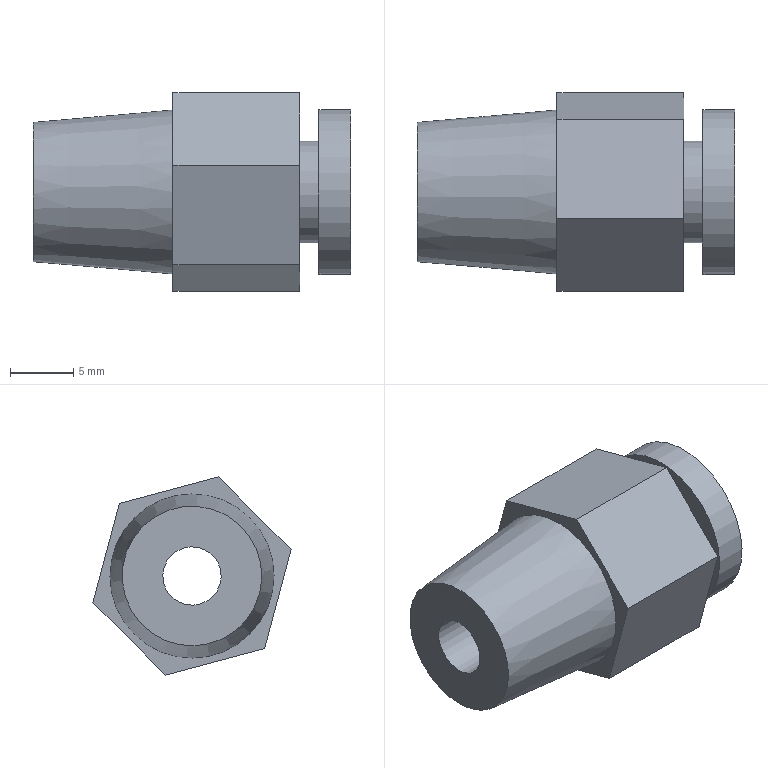Part | NX | features solid 2 | 1 solid | 17 faces | box 25 x 15.612 x 15.618 mm | volume 2729 mm3 | plane 12 | cylinder 4 | cone 1 | commonest cylinder face diameters 4.6 x1 6 x1 8 x1 13 x1
STEP:
#1=CARTESIAN_POINT('',(56.,-265.281,333.212));
#2=VERTEX_POINT('',#1);
#3=CARTESIAN_POINT('',(56.,-273.087,335.309));
#4=VERTEX_POINT('',#3);
#5=CARTESIAN_POINT('',(56.,-265.281,333.212));
#6=DIRECTION('',(0.,-0.9658,0.2594));
#7=VECTOR('',#6,1000.);
#8=LINE('',#5,#7);
#9=EDGE_CURVE('',#2,#4,#8,.T.);
#10=ORIENTED_EDGE('',*,*,#9,.T.);
#11=CARTESIAN_POINT('',(66.,-273.087,335.309));
#12=VERTEX_POINT('',#11);
#13=CARTESIAN_POINT('',(70.,-273.087,335.309));
#14=DIRECTION('',(-1.,0.,0.));
#15=VECTOR('',#14,1000.);
#16=LINE('',#13,#15);
#17=EDGE_CURVE('',#12,#4,#16,.T.);
#18=ORIENTED_EDGE('',*,*,#17,.F.);
#19=CARTESIAN_POINT('',(66.,-265.281,333.212));
#20=VERTEX_POINT('',#19);
#21=CARTESIAN_POINT('',(66.,-265.281,333.212));
#22=DIRECTION('',(0.,-0.9658,0.2594));
#23=VECTOR('',#22,1000.);
#24=LINE('',#21,#23);
#25=EDGE_CURVE('',#20,#12,#24,.T.);
#26=ORIENTED_EDGE('',*,*,#25,.F.);
#27=CARTESIAN_POINT('',(70.,-265.281,333.212));
#28=DIRECTION('',(-1.,0.,0.));
#29=VECTOR('',#28,1000.);
#30=LINE('',#27,#29);
#31=EDGE_CURVE('',#20,#2,#30,.T.);
#32=ORIENTED_EDGE('',*,*,#31,.T.);
#33=EDGE_LOOP('',(#10,#18,#26,#32));
#34=FACE_BOUND('',#33,.T.);
#35=CARTESIAN_POINT('',(70.,-265.281,333.212));
#36=DIRECTION('',(0.,0.2594,0.9658));
#37=DIRECTION('',(0.,-0.9658,0.2594));
#38=AXIS2_PLACEMENT_3D('',#35,#36,#37);
#39=PLANE('',#38);
#40=ADVANCED_FACE('',(#34),#39,.T.);
#41=CARTESIAN_POINT('',(56.,-278.806,329.597));
#42=VERTEX_POINT('',#41);
#43=CARTESIAN_POINT('',(56.,-273.087,335.309));
#44=DIRECTION('',(0.,-0.7076,-0.7066));
#45=VECTOR('',#44,1000.);
#46=LINE('',#43,#45);
#47=EDGE_CURVE('',#4,#42,#46,.T.);
#48=ORIENTED_EDGE('',*,*,#47,.T.);
#49=CARTESIAN_POINT('',(66.,-278.806,329.597));
#50=VERTEX_POINT('',#49);
#51=CARTESIAN_POINT('',(70.,-278.806,329.597));
#52=DIRECTION('',(-1.,0.,0.));
#53=VECTOR('',#52,1000.);
#54=LINE('',#51,#53);
#55=EDGE_CURVE('',#50,#42,#54,.T.);
#56=ORIENTED_EDGE('',*,*,#55,.F.);
#57=CARTESIAN_POINT('',(66.,-273.087,335.309));
#58=DIRECTION('',(0.,-0.7076,-0.7066));
#59=VECTOR('',#58,1000.);
#60=LINE('',#57,#59);
#61=EDGE_CURVE('',#12,#50,#60,.T.);
#62=ORIENTED_EDGE('',*,*,#61,.F.);
#63=ORIENTED_EDGE('',*,*,#17,.T.);
#64=EDGE_LOOP('',(#48,#56,#62,#63));
#65=FACE_BOUND('',#64,.T.);
#66=CARTESIAN_POINT('',(70.,-273.087,335.309));
#67=DIRECTION('',(0.,-0.7066,0.7076));
#68=DIRECTION('',(0.,-0.7076,-0.7066));
#69=AXIS2_PLACEMENT_3D('',#66,#67,#68);
#70=PLANE('',#69);
#71=ADVANCED_FACE('',(#65),#70,.T.);
#72=CARTESIAN_POINT('',(56.,-276.719,321.788));
#73=VERTEX_POINT('',#72);
#74=CARTESIAN_POINT('',(56.,-278.806,329.597));
#75=DIRECTION('',(0.,0.2582,-0.9661));
#76=VECTOR('',#75,1000.);
#77=LINE('',#74,#76);
#78=EDGE_CURVE('',#42,#73,#77,.T.);
#79=ORIENTED_EDGE('',*,*,#78,.T.);
#80=CARTESIAN_POINT('',(66.,-276.719,321.788));
#81=VERTEX_POINT('',#80);
#82=CARTESIAN_POINT('',(70.,-276.719,321.788));
#83=DIRECTION('',(-1.,0.,0.));
#84=VECTOR('',#83,1000.);
#85=LINE('',#82,#84);
#86=EDGE_CURVE('',#81,#73,#85,.T.);
#87=ORIENTED_EDGE('',*,*,#86,.F.);
#88=CARTESIAN_POINT('',(66.,-278.806,329.597));
#89=DIRECTION('',(0.,0.2582,-0.9661));
#90=VECTOR('',#89,1000.);
#91=LINE('',#88,#90);
#92=EDGE_CURVE('',#50,#81,#91,.T.);
#93=ORIENTED_EDGE('',*,*,#92,.F.);
#94=ORIENTED_EDGE('',*,*,#55,.T.);
#95=EDGE_LOOP('',(#79,#87,#93,#94));
#96=FACE_BOUND('',#95,.T.);
#97=CARTESIAN_POINT('',(70.,-278.806,329.597));
#98=DIRECTION('',(0.,-0.9661,-0.2582));
#99=DIRECTION('',(0.,0.2582,-0.9661));
#100=AXIS2_PLACEMENT_3D('',#97,#98,#99);
#101=PLANE('',#100);
#102=ADVANCED_FACE('',(#96),#101,.T.);
#103=CARTESIAN_POINT('',(56.,-268.913,319.691));
#104=VERTEX_POINT('',#103);
#105=CARTESIAN_POINT('',(56.,-276.719,321.788));
#106=DIRECTION('',(0.,0.9658,-0.2594));
#107=VECTOR('',#106,1000.);
#108=LINE('',#105,#107);
#109=EDGE_CURVE('',#73,#104,#108,.T.);
#110=ORIENTED_EDGE('',*,*,#109,.T.);
#111=CARTESIAN_POINT('',(66.,-268.913,319.691));
#112=VERTEX_POINT('',#111);
#113=CARTESIAN_POINT('',(70.,-268.913,319.691));
#114=DIRECTION('',(-1.,0.,0.));
#115=VECTOR('',#114,1000.);
#116=LINE('',#113,#115);
#117=EDGE_CURVE('',#112,#104,#116,.T.);
#118=ORIENTED_EDGE('',*,*,#117,.F.);
#119=CARTESIAN_POINT('',(66.,-276.719,321.788));
#120=DIRECTION('',(0.,0.9658,-0.2594));
#121=VECTOR('',#120,1000.);
#122=LINE('',#119,#121);
#123=EDGE_CURVE('',#81,#112,#122,.T.);
#124=ORIENTED_EDGE('',*,*,#123,.F.);
#125=ORIENTED_EDGE('',*,*,#86,.T.);
#126=EDGE_LOOP('',(#110,#118,#124,#125));
#127=FACE_BOUND('',#126,.T.);
#128=CARTESIAN_POINT('',(70.,-276.719,321.788));
#129=DIRECTION('',(0.,-0.2594,-0.9658));
#130=DIRECTION('',(0.,0.9658,-0.2594));
#131=AXIS2_PLACEMENT_3D('',#128,#129,#130);
#132=PLANE('',#131);
#133=ADVANCED_FACE('',(#127),#132,.T.);
#134=CARTESIAN_POINT('',(56.,-263.194,325.403));
#135=VERTEX_POINT('',#134);
#136=CARTESIAN_POINT('',(56.,-268.913,319.691));
#137=DIRECTION('',(0.,0.7076,0.7066));
#138=VECTOR('',#137,1000.);
#139=LINE('',#136,#138);
#140=EDGE_CURVE('',#104,#135,#139,.T.);
#141=ORIENTED_EDGE('',*,*,#140,.T.);
#142=CARTESIAN_POINT('',(66.,-263.194,325.403));
#143=VERTEX_POINT('',#142);
#144=CARTESIAN_POINT('',(70.,-263.194,325.403));
#145=DIRECTION('',(-1.,0.,0.));
#146=VECTOR('',#145,1000.);
#147=LINE('',#144,#146);
#148=EDGE_CURVE('',#143,#135,#147,.T.);
#149=ORIENTED_EDGE('',*,*,#148,.F.);
#150=CARTESIAN_POINT('',(66.,-268.913,319.691));
#151=DIRECTION('',(0.,0.7076,0.7066));
#152=VECTOR('',#151,1000.);
#153=LINE('',#150,#152);
#154=EDGE_CURVE('',#112,#143,#153,.T.);
#155=ORIENTED_EDGE('',*,*,#154,.F.);
#156=ORIENTED_EDGE('',*,*,#117,.T.);
#157=EDGE_LOOP('',(#141,#149,#155,#156));
#158=FACE_BOUND('',#157,.T.);
#159=CARTESIAN_POINT('',(70.,-268.913,319.691));
#160=DIRECTION('',(0.,0.7066,-0.7076));
#161=DIRECTION('',(0.,0.7076,0.7066));
#162=AXIS2_PLACEMENT_3D('',#159,#160,#161);
#163=PLANE('',#162);
#164=ADVANCED_FACE('',(#158),#163,.T.);
#165=CARTESIAN_POINT('',(56.,-263.194,325.403));
#166=DIRECTION('',(0.,-0.2582,0.9661));
#167=VECTOR('',#166,1000.);
#168=LINE('',#165,#167);
#169=EDGE_CURVE('',#135,#2,#168,.T.);
#170=ORIENTED_EDGE('',*,*,#169,.T.);
#171=ORIENTED_EDGE('',*,*,#31,.F.);
#172=CARTESIAN_POINT('',(66.,-263.194,325.403));
#173=DIRECTION('',(0.,-0.2582,0.9661));
#174=VECTOR('',#173,1000.);
#175=LINE('',#172,#174);
#176=EDGE_CURVE('',#143,#20,#175,.T.);
#177=ORIENTED_EDGE('',*,*,#176,.F.);
#178=ORIENTED_EDGE('',*,*,#148,.T.);
#179=EDGE_LOOP('',(#170,#171,#177,#178));
#180=FACE_BOUND('',#179,.T.);
#181=CARTESIAN_POINT('',(70.,-263.194,325.403));
#182=DIRECTION('',(0.,0.9661,0.2582));
#183=DIRECTION('',(0.,-0.2582,0.9661));
#184=AXIS2_PLACEMENT_3D('',#181,#182,#183);
#185=PLANE('',#184);
#186=ADVANCED_FACE('',(#180),#185,.T.);
#187=ORIENTED_EDGE('',*,*,#25,.T.);
#188=ORIENTED_EDGE('',*,*,#61,.T.);
#189=ORIENTED_EDGE('',*,*,#92,.T.);
#190=ORIENTED_EDGE('',*,*,#123,.T.);
#191=ORIENTED_EDGE('',*,*,#154,.T.);
#192=ORIENTED_EDGE('',*,*,#176,.T.);
#193=EDGE_LOOP('',(#187,#188,#189,#190,#191,#192));
#194=FACE_BOUND('',#193,.T.);
#195=CARTESIAN_POINT('',(66.,-273.83,324.673));
#196=VERTEX_POINT('',#195);
#197=CARTESIAN_POINT('',(66.,-271.,327.5));
#198=DIRECTION('',(-1.,0.,0.));
#199=DIRECTION('',(0.,-0.7076,-0.7066));
#200=AXIS2_PLACEMENT_3D('',#197,#198,#199);
#201=CIRCLE('',#200,4.);
#202=EDGE_CURVE('',#196,#196,#201,.F.);
#203=ORIENTED_EDGE('',*,*,#202,.F.);
#204=EDGE_LOOP('',(#203));
#205=FACE_BOUND('',#204,.T.);
#206=CARTESIAN_POINT('',(66.,-257.475,331.115));
#207=DIRECTION('',(1.,0.,0.));
#208=DIRECTION('',(0.,-0.7076,-0.7066));
#209=AXIS2_PLACEMENT_3D('',#206,#207,#208);
#210=PLANE('',#209);
#211=ADVANCED_FACE('',(#194,#205),#210,.T.);
#212=CARTESIAN_POINT('',(56.,-275.571,322.935));
#213=VERTEX_POINT('',#212);
#214=CARTESIAN_POINT('',(56.,-271.,327.5));
#215=DIRECTION('',(-1.,0.,0.));
#216=DIRECTION('',(0.,-0.7076,-0.7066));
#217=AXIS2_PLACEMENT_3D('',#214,#215,#216);
#218=CIRCLE('',#217,6.46);
#219=EDGE_CURVE('',#213,#213,#218,.F.);
#220=ORIENTED_EDGE('',*,*,#219,.T.);
#221=EDGE_LOOP('',(#220));
#222=FACE_BOUND('',#221,.T.);
#223=ORIENTED_EDGE('',*,*,#9,.F.);
#224=ORIENTED_EDGE('',*,*,#169,.F.);
#225=ORIENTED_EDGE('',*,*,#140,.F.);
#226=ORIENTED_EDGE('',*,*,#109,.F.);
#227=ORIENTED_EDGE('',*,*,#78,.F.);
#228=ORIENTED_EDGE('',*,*,#47,.F.);
#229=EDGE_LOOP('',(#223,#224,#225,#226,#227,#228));
#230=FACE_BOUND('',#229,.T.);
#231=CARTESIAN_POINT('',(56.,-257.475,331.115));
#232=DIRECTION('',(1.,0.,0.));
#233=DIRECTION('',(0.,-0.7076,-0.7066));
#234=AXIS2_PLACEMENT_3D('',#231,#232,#233);
#235=PLANE('',#234);
#236=ADVANCED_FACE('',(#222,#230),#235,.F.);
#237=CARTESIAN_POINT('',(45.,-272.627,325.875));
#238=VERTEX_POINT('',#237);
#239=CARTESIAN_POINT('',(45.,-271.,327.5));
#240=DIRECTION('',(-1.,0.,0.));
#241=DIRECTION('',(0.,-0.7076,-0.7066));
#242=AXIS2_PLACEMENT_3D('',#239,#240,#241);
#243=CIRCLE('',#242,2.3);
#244=EDGE_CURVE('',#238,#238,#243,.T.);
#245=ORIENTED_EDGE('',*,*,#244,.F.);
#246=EDGE_LOOP('',(#245));
#247=FACE_BOUND('',#246,.T.);
#248=CARTESIAN_POINT('',(45.,-267.11,331.385));
#249=VERTEX_POINT('',#248);
#250=CARTESIAN_POINT('',(45.,-271.,327.5));
#251=DIRECTION('',(1.,0.,0.));
#252=DIRECTION('',(0.,0.7076,0.7066));
#253=AXIS2_PLACEMENT_3D('',#250,#251,#252);
#254=CIRCLE('',#253,5.498);
#255=EDGE_CURVE('',#249,#249,#254,.T.);
#256=ORIENTED_EDGE('',*,*,#255,.F.);
#257=EDGE_LOOP('',(#256));
#258=FACE_BOUND('',#257,.T.);
#259=CARTESIAN_POINT('',(45.,-271.,327.5));
#260=DIRECTION('',(-1.,0.,0.));
#261=DIRECTION('',(0.,0.7076,0.7066));
#262=AXIS2_PLACEMENT_3D('',#259,#260,#261);
#263=PLANE('',#262);
#264=ADVANCED_FACE('',(#247,#258),#263,.T.);
#265=ORIENTED_EDGE('',*,*,#255,.T.);
#266=EDGE_LOOP('',(#265));
#267=FACE_BOUND('',#266,.T.);
#268=ORIENTED_EDGE('',*,*,#219,.F.);
#269=EDGE_LOOP('',(#268));
#270=FACE_BOUND('',#269,.T.);
#271=CARTESIAN_POINT('',(45.044,-271.,327.5));
#272=DIRECTION('',(1.,0.,0.));
#273=DIRECTION('',(0.,0.7076,0.7066));
#274=AXIS2_PLACEMENT_3D('',#271,#272,#273);
#275=CONICAL_SURFACE('',#274,5.502,0.08727);
#276=ADVANCED_FACE('',(#267,#270),#275,.T.);
#277=CARTESIAN_POINT('',(53.,-269.373,329.125));
#278=VERTEX_POINT('',#277);
#279=CARTESIAN_POINT('',(53.,-271.,327.5));
#280=DIRECTION('',(1.,0.,0.));
#281=DIRECTION('',(0.,0.7076,0.7066));
#282=AXIS2_PLACEMENT_3D('',#279,#280,#281);
#283=CIRCLE('',#282,2.3);
#284=EDGE_CURVE('',#278,#278,#283,.F.);
#285=ORIENTED_EDGE('',*,*,#284,.F.);
#286=EDGE_LOOP('',(#285));
#287=FACE_BOUND('',#286,.T.);
#288=ORIENTED_EDGE('',*,*,#244,.T.);
#289=EDGE_LOOP('',(#288));
#290=FACE_BOUND('',#289,.T.);
#291=CARTESIAN_POINT('',(45.,-271.,327.5));
#292=DIRECTION('',(1.,0.,0.));
#293=DIRECTION('',(0.,-0.7076,-0.7066));
#294=AXIS2_PLACEMENT_3D('',#291,#292,#293);
#295=CYLINDRICAL_SURFACE('',#294,2.3);
#296=ADVANCED_FACE('',(#287,#290),#295,.F.);
#297=CARTESIAN_POINT('',(53.,-268.877,329.62));
#298=VERTEX_POINT('',#297);
#299=CARTESIAN_POINT('',(53.,-271.,327.5));
#300=DIRECTION('',(1.,0.,0.));
#301=DIRECTION('',(0.,0.7076,0.7066));
#302=AXIS2_PLACEMENT_3D('',#299,#300,#301);
#303=CIRCLE('',#302,3.);
#304=EDGE_CURVE('',#298,#298,#303,.T.);
#305=ORIENTED_EDGE('',*,*,#304,.T.);
#306=EDGE_LOOP('',(#305));
#307=FACE_BOUND('',#306,.T.);
#308=ORIENTED_EDGE('',*,*,#284,.T.);
#309=EDGE_LOOP('',(#308));
#310=FACE_BOUND('',#309,.T.);
#311=CARTESIAN_POINT('',(53.,-271.,327.5));
#312=DIRECTION('',(-1.,0.,0.));
#313=DIRECTION('',(0.,0.7076,0.7066));
#314=AXIS2_PLACEMENT_3D('',#311,#312,#313);
#315=PLANE('',#314);
#316=ADVANCED_FACE('',(#307,#310),#315,.F.);
#317=ORIENTED_EDGE('',*,*,#304,.F.);
#318=EDGE_LOOP('',(#317));
#319=FACE_BOUND('',#318,.T.);
#320=CARTESIAN_POINT('',(70.,-273.123,325.38));
#321=VERTEX_POINT('',#320);
#322=CARTESIAN_POINT('',(70.,-271.,327.5));
#323=DIRECTION('',(1.,0.,0.));
#324=DIRECTION('',(0.,-0.7076,-0.7066));
#325=AXIS2_PLACEMENT_3D('',#322,#323,#324);
#326=CIRCLE('',#325,3.);
#327=EDGE_CURVE('',#321,#321,#326,.T.);
#328=ORIENTED_EDGE('',*,*,#327,.T.);
#329=EDGE_LOOP('',(#328));
#330=FACE_BOUND('',#329,.T.);
#331=CARTESIAN_POINT('',(70.,-271.,327.5));
#332=DIRECTION('',(-1.,0.,0.));
#333=DIRECTION('',(0.,0.7076,0.7066));
#334=AXIS2_PLACEMENT_3D('',#331,#332,#333);
#335=CYLINDRICAL_SURFACE('',#334,3.);
#336=ADVANCED_FACE('',(#319,#330),#335,.F.);
#337=CARTESIAN_POINT('',(70.,-275.599,322.907));
#338=VERTEX_POINT('',#337);
#339=CARTESIAN_POINT('',(70.,-271.,327.5));
#340=DIRECTION('',(-1.,0.,0.));
#341=DIRECTION('',(0.,-0.7076,-0.7066));
#342=AXIS2_PLACEMENT_3D('',#339,#340,#341);
#343=CIRCLE('',#342,6.5);
#344=EDGE_CURVE('',#338,#338,#343,.F.);
#345=ORIENTED_EDGE('',*,*,#344,.T.);
#346=EDGE_LOOP('',(#345));
#347=FACE_BOUND('',#346,.T.);
#348=ORIENTED_EDGE('',*,*,#327,.F.);
#349=EDGE_LOOP('',(#348));
#350=FACE_BOUND('',#349,.T.);
#351=CARTESIAN_POINT('',(70.,-271.,327.5));
#352=DIRECTION('',(1.,0.,0.));
#353=DIRECTION('',(0.,-0.7076,-0.7066));
#354=AXIS2_PLACEMENT_3D('',#351,#352,#353);
#355=PLANE('',#354);
#356=ADVANCED_FACE('',(#347,#350),#355,.T.);
#357=CARTESIAN_POINT('',(67.5,-275.599,322.907));
#358=VERTEX_POINT('',#357);
#359=CARTESIAN_POINT('',(67.5,-271.,327.5));
#360=DIRECTION('',(-1.,0.,0.));
#361=DIRECTION('',(0.,-0.7076,-0.7066));
#362=AXIS2_PLACEMENT_3D('',#359,#360,#361);
#363=CIRCLE('',#362,6.5);
#364=EDGE_CURVE('',#358,#358,#363,.F.);
#365=ORIENTED_EDGE('',*,*,#364,.T.);
#366=EDGE_LOOP('',(#365));
#367=FACE_BOUND('',#366,.T.);
#368=ORIENTED_EDGE('',*,*,#344,.F.);
#369=EDGE_LOOP('',(#368));
#370=FACE_BOUND('',#369,.T.);
#371=CARTESIAN_POINT('',(70.,-271.,327.5));
#372=DIRECTION('',(-1.,0.,0.));
#373=DIRECTION('',(0.,0.7076,0.7066));
#374=AXIS2_PLACEMENT_3D('',#371,#372,#373);
#375=CYLINDRICAL_SURFACE('',#374,6.5);
#376=ADVANCED_FACE('',(#367,#370),#375,.T.);
#377=ORIENTED_EDGE('',*,*,#364,.F.);
#378=EDGE_LOOP('',(#377));
#379=FACE_BOUND('',#378,.T.);
#380=CARTESIAN_POINT('',(67.5,-273.83,324.673));
#381=VERTEX_POINT('',#380);
#382=CARTESIAN_POINT('',(67.5,-271.,327.5));
#383=DIRECTION('',(-1.,0.,0.));
#384=DIRECTION('',(0.,-0.7076,-0.7066));
#385=AXIS2_PLACEMENT_3D('',#382,#383,#384);
#386=CIRCLE('',#385,4.);
#387=EDGE_CURVE('',#381,#381,#386,.F.);
#388=ORIENTED_EDGE('',*,*,#387,.T.);
#389=EDGE_LOOP('',(#388));
#390=FACE_BOUND('',#389,.T.);
#391=CARTESIAN_POINT('',(67.5,-271.,327.5));
#392=DIRECTION('',(1.,0.,0.));
#393=DIRECTION('',(0.,-0.7076,-0.7066));
#394=AXIS2_PLACEMENT_3D('',#391,#392,#393);
#395=PLANE('',#394);
#396=ADVANCED_FACE('',(#379,#390),#395,.F.);
#397=ORIENTED_EDGE('',*,*,#202,.T.);
#398=EDGE_LOOP('',(#397));
#399=FACE_BOUND('',#398,.T.);
#400=ORIENTED_EDGE('',*,*,#387,.F.);
#401=EDGE_LOOP('',(#400));
#402=FACE_BOUND('',#401,.T.);
#403=CARTESIAN_POINT('',(67.5,-271.,327.5));
#404=DIRECTION('',(-1.,0.,0.));
#405=DIRECTION('',(0.,0.7076,0.7066));
#406=AXIS2_PLACEMENT_3D('',#403,#404,#405);
#407=CYLINDRICAL_SURFACE('',#406,4.);
#408=ADVANCED_FACE('',(#399,#402),#407,.T.);
#409=CLOSED_SHELL('',(#40,#71,#102,#133,#164,#186,#211,#236,#264,#276,#296,#316,#336,#356,#376,#396,#408));
#410=MANIFOLD_SOLID_BREP('',#409);
#411=(LENGTH_UNIT()NAMED_UNIT(*)SI_UNIT(.MILLI.,.METRE.));
#412=UNCERTAINTY_MEASURE_WITH_UNIT(LENGTH_MEASURE(0.00001),#411,'','');
#413=(NAMED_UNIT(*)PLANE_ANGLE_UNIT()SI_UNIT($,.RADIAN.));
#414=(NAMED_UNIT(*)SI_UNIT($,.STERADIAN.)SOLID_ANGLE_UNIT());
#415=(GEOMETRIC_REPRESENTATION_CONTEXT(3)GLOBAL_UNCERTAINTY_ASSIGNED_CONTEXT((#412))GLOBAL_UNIT_ASSIGNED_CONTEXT((#411,#413,#414))REPRESENTATION_CONTEXT('',''));
#416=ADVANCED_BREP_SHAPE_REPRESENTATION('',(#410),#415);